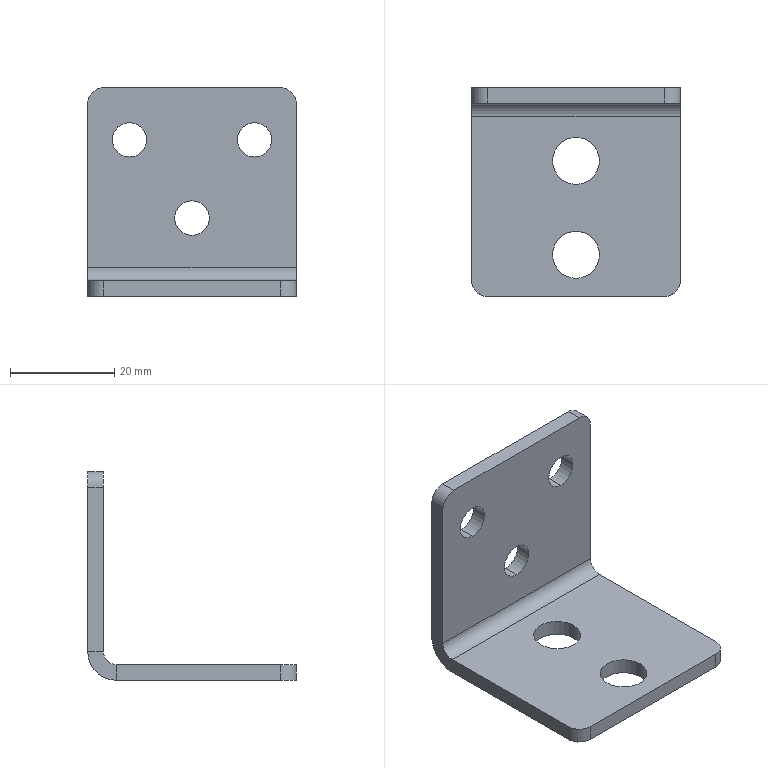Part | STEP file | 1 solid | 28 faces | box 40 x 40 x 40 mm | volume 8321 mm3 | cylinder 16 | plane 12 | commonest cylinder face diameters 6.6 x6 6 x4 9 x4 5 x1 11 x1